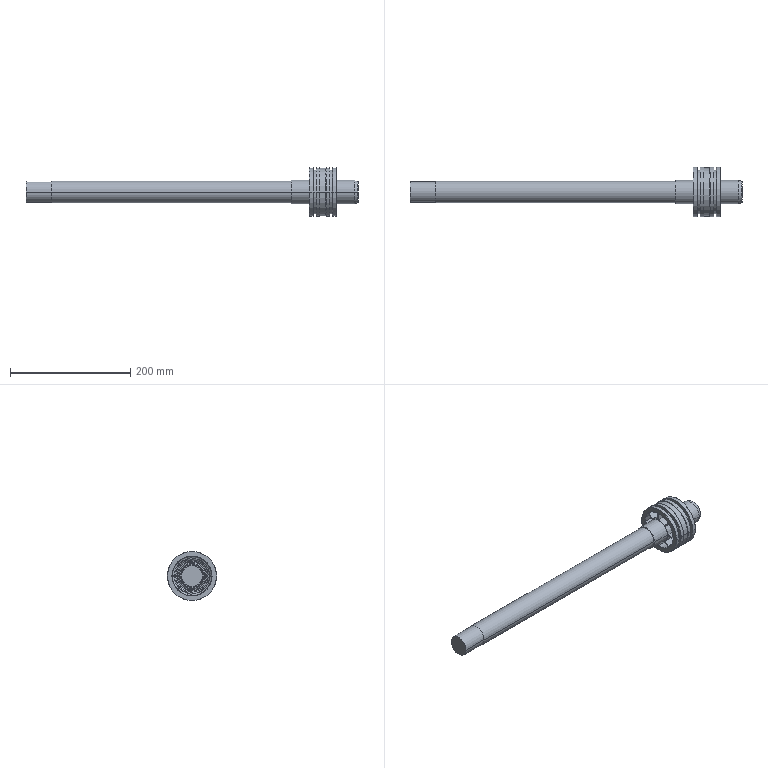Part | STEP file | SCT_80x100x25_r1 | 1 solid | 219 faces | box 553 x 82.1 x 82.1 mm | volume 687780 mm3 | plane 89 | torus 62 | cone 46 | cylinder 22 | commonest cylinder face diameters 82.1 x8 39.1 x4 73.1 x4 35 x2 36 x2 80 x2